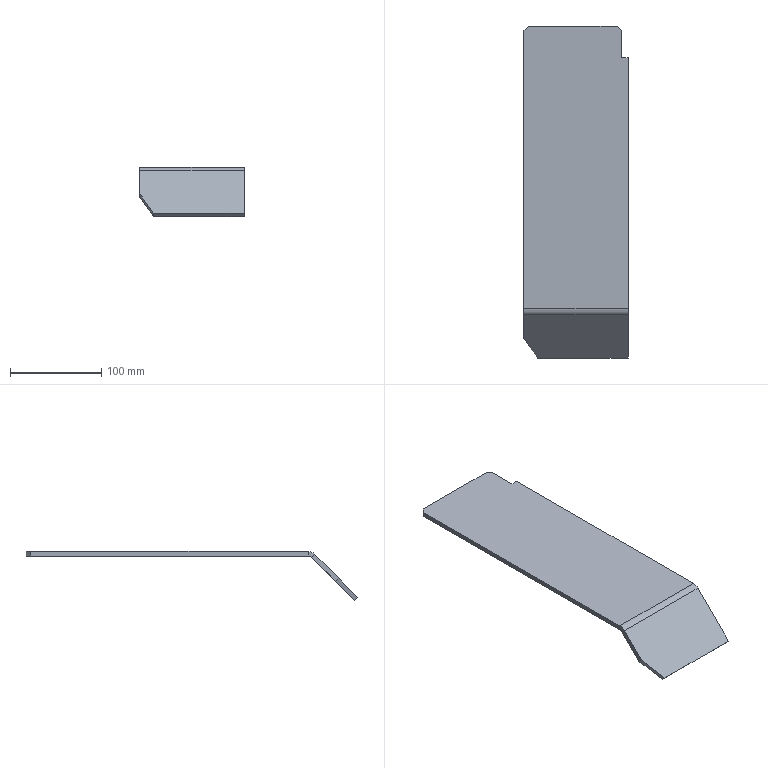Part | STEP file | VD-SYL0380DJ1006_1_1-7_VD-SYL03 | 1 solid | 19 faces | box 114 x 363.205 x 53.74 mm | volume 215041 mm3 | plane 17 | cylinder 2 | commonest cylinder face diameters 10 x1 20 x1
STEP:
#1=CARTESIAN_POINT('',(45.,156.5,0.));
#2=VERTEX_POINT('',#1);
#3=CARTESIAN_POINT('',(50.,151.5,0.));
#4=VERTEX_POINT('',#3);
#5=CARTESIAN_POINT('',(45.,156.5,0.));
#6=DIRECTION('',(0.7071,-0.7071,0.));
#7=VECTOR('',#6,1000.);
#8=LINE('',#5,#7);
#9=EDGE_CURVE('',#2,#4,#8,.T.);
#10=ORIENTED_EDGE('',*,*,#9,.T.);
#11=CARTESIAN_POINT('',(50.,121.5,0.));
#12=VERTEX_POINT('',#11);
#13=CARTESIAN_POINT('',(50.,121.5,0.));
#14=DIRECTION('',(0.,1.,0.));
#15=VECTOR('',#14,1000.);
#16=LINE('',#13,#15);
#17=EDGE_CURVE('',#12,#4,#16,.T.);
#18=ORIENTED_EDGE('',*,*,#17,.F.);
#19=CARTESIAN_POINT('',(57.,121.5,0.));
#20=VERTEX_POINT('',#19);
#21=CARTESIAN_POINT('',(50.,121.5,0.));
#22=DIRECTION('',(1.,0.,0.));
#23=VECTOR('',#22,1000.);
#24=LINE('',#21,#23);
#25=EDGE_CURVE('',#12,#20,#24,.T.);
#26=ORIENTED_EDGE('',*,*,#25,.T.);
#27=CARTESIAN_POINT('',(57.,-152.358,0.));
#28=VERTEX_POINT('',#27);
#29=CARTESIAN_POINT('',(57.,121.5,0.));
#30=DIRECTION('',(0.,-1.,0.));
#31=VECTOR('',#30,1000.);
#32=LINE('',#29,#31);
#33=EDGE_CURVE('',#20,#28,#32,.T.);
#34=ORIENTED_EDGE('',*,*,#33,.T.);
#35=CARTESIAN_POINT('',(-57.,-152.358,0.));
#36=VERTEX_POINT('',#35);
#37=CARTESIAN_POINT('',(-57.,-152.358,0.));
#38=DIRECTION('',(1.,0.,0.));
#39=VECTOR('',#38,1000.);
#40=LINE('',#37,#39);
#41=EDGE_CURVE('',#36,#28,#40,.T.);
#42=ORIENTED_EDGE('',*,*,#41,.F.);
#43=CARTESIAN_POINT('',(-57.,151.5,0.));
#44=VERTEX_POINT('',#43);
#45=CARTESIAN_POINT('',(-57.,-152.358,0.));
#46=DIRECTION('',(0.,1.,0.));
#47=VECTOR('',#46,1000.);
#48=LINE('',#45,#47);
#49=EDGE_CURVE('',#36,#44,#48,.T.);
#50=ORIENTED_EDGE('',*,*,#49,.T.);
#51=CARTESIAN_POINT('',(-52.,156.5,0.));
#52=VERTEX_POINT('',#51);
#53=CARTESIAN_POINT('',(-57.,151.5,0.));
#54=DIRECTION('',(0.7071,0.7071,0.));
#55=VECTOR('',#54,1000.);
#56=LINE('',#53,#55);
#57=EDGE_CURVE('',#44,#52,#56,.T.);
#58=ORIENTED_EDGE('',*,*,#57,.T.);
#59=CARTESIAN_POINT('',(-52.,156.5,0.));
#60=DIRECTION('',(1.,0.,0.));
#61=VECTOR('',#60,1000.);
#62=LINE('',#59,#61);
#63=EDGE_CURVE('',#52,#2,#62,.T.);
#64=ORIENTED_EDGE('',*,*,#63,.T.);
#65=EDGE_LOOP('',(#10,#18,#26,#34,#42,#50,#58,#64));
#66=FACE_OUTER_BOUND('',#65,.T.);
#67=CARTESIAN_POINT('',(0.,0.,0.));
#68=DIRECTION('',(0.,0.,1.));
#69=DIRECTION('',(1.,0.,0.));
#70=AXIS2_PLACEMENT_3D('',#67,#68,#69);
#71=PLANE('',#70);
#72=ADVANCED_FACE('',(#66),#71,.F.);
#73=CARTESIAN_POINT('',(-57.,-185.491,-23.991));
#74=VERTEX_POINT('',#73);
#75=CARTESIAN_POINT('',(-42.,-206.705,-45.205));
#76=VERTEX_POINT('',#75);
#77=CARTESIAN_POINT('',(-57.,-185.491,-23.991));
#78=DIRECTION('',(0.4472,-0.6325,-0.6325));
#79=VECTOR('',#78,1000.);
#80=LINE('',#77,#79);
#81=EDGE_CURVE('',#74,#76,#80,.T.);
#82=ORIENTED_EDGE('',*,*,#81,.T.);
#83=CARTESIAN_POINT('',(57.,-206.705,-45.205));
#84=VERTEX_POINT('',#83);
#85=CARTESIAN_POINT('',(-42.,-206.705,-45.205));
#86=DIRECTION('',(1.,0.,0.));
#87=VECTOR('',#86,1000.);
#88=LINE('',#85,#87);
#89=EDGE_CURVE('',#76,#84,#88,.T.);
#90=ORIENTED_EDGE('',*,*,#89,.T.);
#91=CARTESIAN_POINT('',(57.,-159.429,2.071));
#92=VERTEX_POINT('',#91);
#93=CARTESIAN_POINT('',(57.,-159.429,2.071));
#94=DIRECTION('',(0.,-0.7071,-0.7071));
#95=VECTOR('',#94,1000.);
#96=LINE('',#93,#95);
#97=EDGE_CURVE('',#92,#84,#96,.T.);
#98=ORIENTED_EDGE('',*,*,#97,.F.);
#99=CARTESIAN_POINT('',(-57.,-159.429,2.071));
#100=VERTEX_POINT('',#99);
#101=CARTESIAN_POINT('',(-57.,-159.429,2.071));
#102=DIRECTION('',(1.,0.,0.));
#103=VECTOR('',#102,1000.);
#104=LINE('',#101,#103);
#105=EDGE_CURVE('',#100,#92,#104,.T.);
#106=ORIENTED_EDGE('',*,*,#105,.F.);
#107=CARTESIAN_POINT('',(-57.,-185.491,-23.991));
#108=DIRECTION('',(0.,0.7071,0.7071));
#109=VECTOR('',#108,1000.);
#110=LINE('',#107,#109);
#111=EDGE_CURVE('',#74,#100,#110,.T.);
#112=ORIENTED_EDGE('',*,*,#111,.F.);
#113=EDGE_LOOP('',(#82,#90,#98,#106,#112));
#114=FACE_OUTER_BOUND('',#113,.T.);
#115=CARTESIAN_POINT('',(-57.,-156.5,5.));
#116=DIRECTION('',(0.,-0.7071,0.7071));
#117=DIRECTION('',(-1.,0.,0.));
#118=AXIS2_PLACEMENT_3D('',#115,#116,#117);
#119=PLANE('',#118);
#120=ADVANCED_FACE('',(#114),#119,.T.);
#121=ORIENTED_EDGE('',*,*,#105,.T.);
#122=CARTESIAN_POINT('',(57.,-152.358,5.));
#123=VERTEX_POINT('',#122);
#124=CARTESIAN_POINT('',(57.,-152.358,-5.));
#125=DIRECTION('',(1.,0.,0.));
#126=DIRECTION('',(0.,0.,1.));
#127=AXIS2_PLACEMENT_3D('',#124,#125,#126);
#128=CIRCLE('',#127,10.);
#129=EDGE_CURVE('',#123,#92,#128,.T.);
#130=ORIENTED_EDGE('',*,*,#129,.F.);
#131=CARTESIAN_POINT('',(-57.,-152.358,5.));
#132=VERTEX_POINT('',#131);
#133=CARTESIAN_POINT('',(57.,-152.358,5.));
#134=DIRECTION('',(-1.,0.,0.));
#135=VECTOR('',#134,1000.);
#136=LINE('',#133,#135);
#137=EDGE_CURVE('',#123,#132,#136,.T.);
#138=ORIENTED_EDGE('',*,*,#137,.T.);
#139=CARTESIAN_POINT('',(-57.,-152.358,-5.));
#140=DIRECTION('',(-1.,0.,0.));
#141=DIRECTION('',(0.,-0.7071,0.7071));
#142=AXIS2_PLACEMENT_3D('',#139,#140,#141);
#143=CIRCLE('',#142,10.);
#144=EDGE_CURVE('',#100,#132,#143,.T.);
#145=ORIENTED_EDGE('',*,*,#144,.F.);
#146=EDGE_LOOP('',(#121,#130,#138,#145));
#147=FACE_OUTER_BOUND('',#146,.T.);
#148=CARTESIAN_POINT('',(57.,-152.358,-5.));
#149=DIRECTION('',(-1.,0.,0.));
#150=DIRECTION('',(0.,0.,1.));
#151=AXIS2_PLACEMENT_3D('',#148,#149,#150);
#152=CYLINDRICAL_SURFACE('',#151,10.);
#153=ADVANCED_FACE('',(#147),#152,.T.);
#154=CARTESIAN_POINT('',(-52.,156.5,5.));
#155=VERTEX_POINT('',#154);
#156=CARTESIAN_POINT('',(-57.,151.5,5.));
#157=VERTEX_POINT('',#156);
#158=CARTESIAN_POINT('',(-52.,156.5,5.));
#159=DIRECTION('',(-0.7071,-0.7071,0.));
#160=VECTOR('',#159,1000.);
#161=LINE('',#158,#160);
#162=EDGE_CURVE('',#155,#157,#161,.T.);
#163=ORIENTED_EDGE('',*,*,#162,.T.);
#164=CARTESIAN_POINT('',(-57.,-152.358,5.));
#165=DIRECTION('',(0.,1.,0.));
#166=VECTOR('',#165,1000.);
#167=LINE('',#164,#166);
#168=EDGE_CURVE('',#132,#157,#167,.T.);
#169=ORIENTED_EDGE('',*,*,#168,.F.);
#170=ORIENTED_EDGE('',*,*,#137,.F.);
#171=CARTESIAN_POINT('',(57.,121.5,5.));
#172=VERTEX_POINT('',#171);
#173=CARTESIAN_POINT('',(57.,121.5,5.));
#174=DIRECTION('',(0.,-1.,0.));
#175=VECTOR('',#174,1000.);
#176=LINE('',#173,#175);
#177=EDGE_CURVE('',#172,#123,#176,.T.);
#178=ORIENTED_EDGE('',*,*,#177,.F.);
#179=CARTESIAN_POINT('',(50.,121.5,5.));
#180=VERTEX_POINT('',#179);
#181=CARTESIAN_POINT('',(50.,121.5,5.));
#182=DIRECTION('',(1.,0.,0.));
#183=VECTOR('',#182,1000.);
#184=LINE('',#181,#183);
#185=EDGE_CURVE('',#180,#172,#184,.T.);
#186=ORIENTED_EDGE('',*,*,#185,.F.);
#187=CARTESIAN_POINT('',(50.,151.5,5.));
#188=VERTEX_POINT('',#187);
#189=CARTESIAN_POINT('',(50.,121.5,5.));
#190=DIRECTION('',(0.,1.,0.));
#191=VECTOR('',#190,1000.);
#192=LINE('',#189,#191);
#193=EDGE_CURVE('',#180,#188,#192,.T.);
#194=ORIENTED_EDGE('',*,*,#193,.T.);
#195=CARTESIAN_POINT('',(45.,156.5,5.));
#196=VERTEX_POINT('',#195);
#197=CARTESIAN_POINT('',(50.,151.5,5.));
#198=DIRECTION('',(-0.7071,0.7071,0.));
#199=VECTOR('',#198,1000.);
#200=LINE('',#197,#199);
#201=EDGE_CURVE('',#188,#196,#200,.T.);
#202=ORIENTED_EDGE('',*,*,#201,.T.);
#203=CARTESIAN_POINT('',(-52.,156.5,5.));
#204=DIRECTION('',(1.,0.,0.));
#205=VECTOR('',#204,1000.);
#206=LINE('',#203,#205);
#207=EDGE_CURVE('',#155,#196,#206,.T.);
#208=ORIENTED_EDGE('',*,*,#207,.F.);
#209=EDGE_LOOP('',(#163,#169,#170,#178,#186,#194,#202,#208));
#210=FACE_OUTER_BOUND('',#209,.T.);
#211=CARTESIAN_POINT('',(0.,0.,5.));
#212=DIRECTION('',(0.,0.,1.));
#213=DIRECTION('',(1.,0.,0.));
#214=AXIS2_PLACEMENT_3D('',#211,#212,#213);
#215=PLANE('',#214);
#216=ADVANCED_FACE('',(#210),#215,.T.);
#217=ORIENTED_EDGE('',*,*,#25,.F.);
#218=CARTESIAN_POINT('',(50.,121.5,5.));
#219=DIRECTION('',(0.,0.,-1.));
#220=VECTOR('',#219,1000.);
#221=LINE('',#218,#220);
#222=EDGE_CURVE('',#180,#12,#221,.T.);
#223=ORIENTED_EDGE('',*,*,#222,.F.);
#224=ORIENTED_EDGE('',*,*,#185,.T.);
#225=CARTESIAN_POINT('',(57.,121.5,5.));
#226=DIRECTION('',(0.,0.,-1.));
#227=VECTOR('',#226,1000.);
#228=LINE('',#225,#227);
#229=EDGE_CURVE('',#172,#20,#228,.T.);
#230=ORIENTED_EDGE('',*,*,#229,.T.);
#231=EDGE_LOOP('',(#217,#223,#224,#230));
#232=FACE_OUTER_BOUND('',#231,.T.);
#233=CARTESIAN_POINT('',(53.5,121.5,5.));
#234=DIRECTION('',(0.,-1.,0.));
#235=DIRECTION('',(0.,0.,-1.));
#236=AXIS2_PLACEMENT_3D('',#233,#234,#235);
#237=PLANE('',#236);
#238=ADVANCED_FACE('',(#232),#237,.F.);
#239=ORIENTED_EDGE('',*,*,#17,.T.);
#240=CARTESIAN_POINT('',(50.,151.5,5.));
#241=DIRECTION('',(0.,0.,-1.));
#242=VECTOR('',#241,1000.);
#243=LINE('',#240,#242);
#244=EDGE_CURVE('',#188,#4,#243,.T.);
#245=ORIENTED_EDGE('',*,*,#244,.F.);
#246=ORIENTED_EDGE('',*,*,#193,.F.);
#247=ORIENTED_EDGE('',*,*,#222,.T.);
#248=EDGE_LOOP('',(#239,#245,#246,#247));
#249=FACE_OUTER_BOUND('',#248,.T.);
#250=CARTESIAN_POINT('',(50.,139.,5.));
#251=DIRECTION('',(1.,0.,0.));
#252=DIRECTION('',(0.,1.,0.));
#253=AXIS2_PLACEMENT_3D('',#250,#251,#252);
#254=PLANE('',#253);
#255=ADVANCED_FACE('',(#249),#254,.T.);
#256=ORIENTED_EDGE('',*,*,#9,.F.);
#257=CARTESIAN_POINT('',(45.,156.5,5.));
#258=DIRECTION('',(0.,0.,-1.));
#259=VECTOR('',#258,1000.);
#260=LINE('',#257,#259);
#261=EDGE_CURVE('',#196,#2,#260,.T.);
#262=ORIENTED_EDGE('',*,*,#261,.F.);
#263=ORIENTED_EDGE('',*,*,#201,.F.);
#264=ORIENTED_EDGE('',*,*,#244,.T.);
#265=EDGE_LOOP('',(#256,#262,#263,#264));
#266=FACE_OUTER_BOUND('',#265,.T.);
#267=CARTESIAN_POINT('',(47.5,154.,5.));
#268=DIRECTION('',(0.7071,0.7071,0.));
#269=DIRECTION('',(0.,0.,-1.));
#270=AXIS2_PLACEMENT_3D('',#267,#268,#269);
#271=PLANE('',#270);
#272=ADVANCED_FACE('',(#266),#271,.T.);
#273=ORIENTED_EDGE('',*,*,#63,.F.);
#274=CARTESIAN_POINT('',(-52.,156.5,5.));
#275=DIRECTION('',(0.,0.,-1.));
#276=VECTOR('',#275,1000.);
#277=LINE('',#274,#276);
#278=EDGE_CURVE('',#155,#52,#277,.T.);
#279=ORIENTED_EDGE('',*,*,#278,.F.);
#280=ORIENTED_EDGE('',*,*,#207,.T.);
#281=ORIENTED_EDGE('',*,*,#261,.T.);
#282=EDGE_LOOP('',(#273,#279,#280,#281));
#283=FACE_OUTER_BOUND('',#282,.T.);
#284=CARTESIAN_POINT('',(0.,156.5,5.));
#285=DIRECTION('',(0.,-1.,0.));
#286=DIRECTION('',(0.,0.,-1.));
#287=AXIS2_PLACEMENT_3D('',#284,#285,#286);
#288=PLANE('',#287);
#289=ADVANCED_FACE('',(#283),#288,.F.);
#290=ORIENTED_EDGE('',*,*,#57,.F.);
#291=CARTESIAN_POINT('',(-57.,151.5,5.));
#292=DIRECTION('',(0.,0.,-1.));
#293=VECTOR('',#292,1000.);
#294=LINE('',#291,#293);
#295=EDGE_CURVE('',#157,#44,#294,.T.);
#296=ORIENTED_EDGE('',*,*,#295,.F.);
#297=ORIENTED_EDGE('',*,*,#162,.F.);
#298=ORIENTED_EDGE('',*,*,#278,.T.);
#299=EDGE_LOOP('',(#290,#296,#297,#298));
#300=FACE_OUTER_BOUND('',#299,.T.);
#301=CARTESIAN_POINT('',(-54.5,154.,5.));
#302=DIRECTION('',(-0.7071,0.7071,0.));
#303=DIRECTION('',(0.,0.,1.));
#304=AXIS2_PLACEMENT_3D('',#301,#302,#303);
#305=PLANE('',#304);
#306=ADVANCED_FACE('',(#300),#305,.T.);
#307=ORIENTED_EDGE('',*,*,#49,.F.);
#308=CARTESIAN_POINT('',(-57.,-152.358,5.));
#309=DIRECTION('',(0.,0.,-1.));
#310=VECTOR('',#309,1000.);
#311=LINE('',#308,#310);
#312=EDGE_CURVE('',#132,#36,#311,.T.);
#313=ORIENTED_EDGE('',*,*,#312,.F.);
#314=ORIENTED_EDGE('',*,*,#168,.T.);
#315=ORIENTED_EDGE('',*,*,#295,.T.);
#316=EDGE_LOOP('',(#307,#313,#314,#315));
#317=FACE_OUTER_BOUND('',#316,.T.);
#318=CARTESIAN_POINT('',(-57.,0.,5.));
#319=DIRECTION('',(1.,0.,0.));
#320=DIRECTION('',(0.,1.,0.));
#321=AXIS2_PLACEMENT_3D('',#318,#319,#320);
#322=PLANE('',#321);
#323=ADVANCED_FACE('',(#317),#322,.F.);
#324=CARTESIAN_POINT('',(-57.,-155.893,-1.464));
#325=VERTEX_POINT('',#324);
#326=CARTESIAN_POINT('',(-57.,-152.358,-5.));
#327=DIRECTION('',(1.,0.,0.));
#328=DIRECTION('',(0.,0.,1.));
#329=AXIS2_PLACEMENT_3D('',#326,#327,#328);
#330=CIRCLE('',#329,5.);
#331=EDGE_CURVE('',#36,#325,#330,.T.);
#332=ORIENTED_EDGE('',*,*,#331,.T.);
#333=CARTESIAN_POINT('',(-57.,-159.429,2.071));
#334=DIRECTION('',(0.,0.7071,-0.7071));
#335=VECTOR('',#334,1000.);
#336=LINE('',#333,#335);
#337=EDGE_CURVE('',#100,#325,#336,.T.);
#338=ORIENTED_EDGE('',*,*,#337,.F.);
#339=ORIENTED_EDGE('',*,*,#144,.T.);
#340=ORIENTED_EDGE('',*,*,#312,.T.);
#341=EDGE_LOOP('',(#332,#338,#339,#340));
#342=FACE_OUTER_BOUND('',#341,.T.);
#343=CARTESIAN_POINT('',(-57.,-152.358,-5.));
#344=DIRECTION('',(1.,0.,0.));
#345=DIRECTION('',(0.,1.,0.));
#346=AXIS2_PLACEMENT_3D('',#343,#344,#345);
#347=PLANE('',#346);
#348=ADVANCED_FACE('',(#342),#347,.F.);
#349=ORIENTED_EDGE('',*,*,#41,.T.);
#350=CARTESIAN_POINT('',(57.,-155.893,-1.464));
#351=VERTEX_POINT('',#350);
#352=CARTESIAN_POINT('',(57.,-152.358,-5.));
#353=DIRECTION('',(-1.,0.,0.));
#354=DIRECTION('',(0.,-0.7071,0.7071));
#355=AXIS2_PLACEMENT_3D('',#352,#353,#354);
#356=CIRCLE('',#355,5.);
#357=EDGE_CURVE('',#351,#28,#356,.T.);
#358=ORIENTED_EDGE('',*,*,#357,.F.);
#359=CARTESIAN_POINT('',(57.,-155.893,-1.464));
#360=DIRECTION('',(-1.,0.,0.));
#361=VECTOR('',#360,1000.);
#362=LINE('',#359,#361);
#363=EDGE_CURVE('',#351,#325,#362,.T.);
#364=ORIENTED_EDGE('',*,*,#363,.T.);
#365=ORIENTED_EDGE('',*,*,#331,.F.);
#366=EDGE_LOOP('',(#349,#358,#364,#365));
#367=FACE_OUTER_BOUND('',#366,.T.);
#368=CARTESIAN_POINT('',(57.,-152.358,-5.));
#369=DIRECTION('',(-1.,0.,0.));
#370=DIRECTION('',(0.,0.,1.));
#371=AXIS2_PLACEMENT_3D('',#368,#369,#370);
#372=CYLINDRICAL_SURFACE('',#371,5.);
#373=ADVANCED_FACE('',(#367),#372,.F.);
#374=ORIENTED_EDGE('',*,*,#363,.F.);
#375=CARTESIAN_POINT('',(57.,-203.169,-48.74));
#376=VERTEX_POINT('',#375);
#377=CARTESIAN_POINT('',(57.,-203.169,-48.74));
#378=DIRECTION('',(0.,0.7071,0.7071));
#379=VECTOR('',#378,1000.);
#380=LINE('',#377,#379);
#381=EDGE_CURVE('',#376,#351,#380,.T.);
#382=ORIENTED_EDGE('',*,*,#381,.F.);
#383=CARTESIAN_POINT('',(-42.,-203.169,-48.74));
#384=VERTEX_POINT('',#383);
#385=CARTESIAN_POINT('',(-42.,-203.169,-48.74));
#386=DIRECTION('',(1.,0.,0.));
#387=VECTOR('',#386,1000.);
#388=LINE('',#385,#387);
#389=EDGE_CURVE('',#384,#376,#388,.T.);
#390=ORIENTED_EDGE('',*,*,#389,.F.);
#391=CARTESIAN_POINT('',(-57.,-181.956,-27.527));
#392=VERTEX_POINT('',#391);
#393=CARTESIAN_POINT('',(-42.,-203.169,-48.74));
#394=DIRECTION('',(-0.4472,0.6325,0.6325));
#395=VECTOR('',#394,1000.);
#396=LINE('',#393,#395);
#397=EDGE_CURVE('',#384,#392,#396,.T.);
#398=ORIENTED_EDGE('',*,*,#397,.T.);
#399=CARTESIAN_POINT('',(-57.,-155.893,-1.464));
#400=DIRECTION('',(0.,-0.7071,-0.7071));
#401=VECTOR('',#400,1000.);
#402=LINE('',#399,#401);
#403=EDGE_CURVE('',#325,#392,#402,.T.);
#404=ORIENTED_EDGE('',*,*,#403,.F.);
#405=EDGE_LOOP('',(#374,#382,#390,#398,#404));
#406=FACE_OUTER_BOUND('',#405,.T.);
#407=CARTESIAN_POINT('',(-57.,-152.964,1.464));
#408=DIRECTION('',(0.,-0.7071,0.7071));
#409=DIRECTION('',(-1.,0.,0.));
#410=AXIS2_PLACEMENT_3D('',#407,#408,#409);
#411=PLANE('',#410);
#412=ADVANCED_FACE('',(#406),#411,.F.);
#413=CARTESIAN_POINT('',(-57.,-181.956,-27.527));
#414=DIRECTION('',(0.,-0.7071,0.7071));
#415=VECTOR('',#414,1000.);
#416=LINE('',#413,#415);
#417=EDGE_CURVE('',#392,#74,#416,.T.);
#418=ORIENTED_EDGE('',*,*,#417,.T.);
#419=ORIENTED_EDGE('',*,*,#111,.T.);
#420=ORIENTED_EDGE('',*,*,#337,.T.);
#421=ORIENTED_EDGE('',*,*,#403,.T.);
#422=EDGE_LOOP('',(#418,#419,#420,#421));
#423=FACE_OUTER_BOUND('',#422,.T.);
#424=CARTESIAN_POINT('',(-57.,-185.491,-23.991));
#425=DIRECTION('',(1.,0.,0.));
#426=DIRECTION('',(0.,1.,0.));
#427=AXIS2_PLACEMENT_3D('',#424,#425,#426);
#428=PLANE('',#427);
#429=ADVANCED_FACE('',(#423),#428,.F.);
#430=ORIENTED_EDGE('',*,*,#397,.F.);
#431=CARTESIAN_POINT('',(-42.,-206.705,-45.205));
#432=DIRECTION('',(0.,0.7071,-0.7071));
#433=VECTOR('',#432,1000.);
#434=LINE('',#431,#433);
#435=EDGE_CURVE('',#76,#384,#434,.T.);
#436=ORIENTED_EDGE('',*,*,#435,.F.);
#437=ORIENTED_EDGE('',*,*,#81,.F.);
#438=ORIENTED_EDGE('',*,*,#417,.F.);
#439=EDGE_LOOP('',(#430,#436,#437,#438));
#440=FACE_OUTER_BOUND('',#439,.T.);
#441=CARTESIAN_POINT('',(-42.,-206.705,-45.205));
#442=DIRECTION('',(0.8944,0.3162,0.3162));
#443=DIRECTION('',(0.,0.7071,-0.7071));
#444=AXIS2_PLACEMENT_3D('',#441,#442,#443);
#445=PLANE('',#444);
#446=ADVANCED_FACE('',(#440),#445,.F.);
#447=ORIENTED_EDGE('',*,*,#389,.T.);
#448=CARTESIAN_POINT('',(57.,-206.705,-45.205));
#449=DIRECTION('',(0.,0.7071,-0.7071));
#450=VECTOR('',#449,1000.);
#451=LINE('',#448,#450);
#452=EDGE_CURVE('',#84,#376,#451,.T.);
#453=ORIENTED_EDGE('',*,*,#452,.F.);
#454=ORIENTED_EDGE('',*,*,#89,.F.);
#455=ORIENTED_EDGE('',*,*,#435,.T.);
#456=EDGE_LOOP('',(#447,#453,#454,#455));
#457=FACE_OUTER_BOUND('',#456,.T.);
#458=CARTESIAN_POINT('',(0.,-206.705,-45.205));
#459=DIRECTION('',(0.,-0.7071,-0.7071));
#460=DIRECTION('',(0.,-0.7071,0.7071));
#461=AXIS2_PLACEMENT_3D('',#458,#459,#460);
#462=PLANE('',#461);
#463=ADVANCED_FACE('',(#457),#462,.T.);
#464=ORIENTED_EDGE('',*,*,#381,.T.);
#465=CARTESIAN_POINT('',(57.,-159.429,2.071));
#466=DIRECTION('',(0.,0.7071,-0.7071));
#467=VECTOR('',#466,1000.);
#468=LINE('',#465,#467);
#469=EDGE_CURVE('',#92,#351,#468,.T.);
#470=ORIENTED_EDGE('',*,*,#469,.F.);
#471=ORIENTED_EDGE('',*,*,#97,.T.);
#472=ORIENTED_EDGE('',*,*,#452,.T.);
#473=EDGE_LOOP('',(#464,#470,#471,#472));
#474=FACE_OUTER_BOUND('',#473,.T.);
#475=CARTESIAN_POINT('',(57.,-159.429,2.071));
#476=DIRECTION('',(-1.,0.,0.));
#477=DIRECTION('',(0.,0.,1.));
#478=AXIS2_PLACEMENT_3D('',#475,#476,#477);
#479=PLANE('',#478);
#480=ADVANCED_FACE('',(#474),#479,.F.);
#481=ORIENTED_EDGE('',*,*,#357,.T.);
#482=CARTESIAN_POINT('',(57.,-152.358,5.));
#483=DIRECTION('',(0.,0.,-1.));
#484=VECTOR('',#483,1000.);
#485=LINE('',#482,#484);
#486=EDGE_CURVE('',#123,#28,#485,.T.);
#487=ORIENTED_EDGE('',*,*,#486,.F.);
#488=ORIENTED_EDGE('',*,*,#129,.T.);
#489=ORIENTED_EDGE('',*,*,#469,.T.);
#490=EDGE_LOOP('',(#481,#487,#488,#489));
#491=FACE_OUTER_BOUND('',#490,.T.);
#492=CARTESIAN_POINT('',(57.,-152.358,-5.));
#493=DIRECTION('',(1.,0.,0.));
#494=DIRECTION('',(0.,1.,0.));
#495=AXIS2_PLACEMENT_3D('',#492,#493,#494);
#496=PLANE('',#495);
#497=ADVANCED_FACE('',(#491),#496,.T.);
#498=ORIENTED_EDGE('',*,*,#33,.F.);
#499=ORIENTED_EDGE('',*,*,#229,.F.);
#500=ORIENTED_EDGE('',*,*,#177,.T.);
#501=ORIENTED_EDGE('',*,*,#486,.T.);
#502=EDGE_LOOP('',(#498,#499,#500,#501));
#503=FACE_OUTER_BOUND('',#502,.T.);
#504=CARTESIAN_POINT('',(57.,0.,5.));
#505=DIRECTION('',(1.,0.,0.));
#506=DIRECTION('',(0.,1.,0.));
#507=AXIS2_PLACEMENT_3D('',#504,#505,#506);
#508=PLANE('',#507);
#509=ADVANCED_FACE('',(#503),#508,.T.);
#510=CLOSED_SHELL('',(#72,#120,#153,#216,#238,#255,#272,#289,#306,#323,#348,#373,#412,#429,#446,#463,#480,#497,#509));
#511=MANIFOLD_SOLID_BREP('',#510);
#512=CARTESIAN_POINT('',(0.,0.,0.));
#513=DIRECTION('',(0.,0.,1.));
#514=DIRECTION('',(1.,0.,0.));
#515=AXIS2_PLACEMENT_3D('',#512,#513,#514);
#516=(LENGTH_UNIT()NAMED_UNIT(*)SI_UNIT(.MILLI.,.METRE.));
#517=UNCERTAINTY_MEASURE_WITH_UNIT(LENGTH_MEASURE(0.00001),#516,'','');
#518=(NAMED_UNIT(*)PLANE_ANGLE_UNIT()SI_UNIT($,.RADIAN.));
#519=(NAMED_UNIT(*)SI_UNIT($,.STERADIAN.)SOLID_ANGLE_UNIT());
#520=(GEOMETRIC_REPRESENTATION_CONTEXT(3)GLOBAL_UNCERTAINTY_ASSIGNED_CONTEXT((#517))GLOBAL_UNIT_ASSIGNED_CONTEXT((#516,#518,#519))REPRESENTATION_CONTEXT('',''));
#521=ADVANCED_BREP_SHAPE_REPRESENTATION('',(#511,#515),#520);